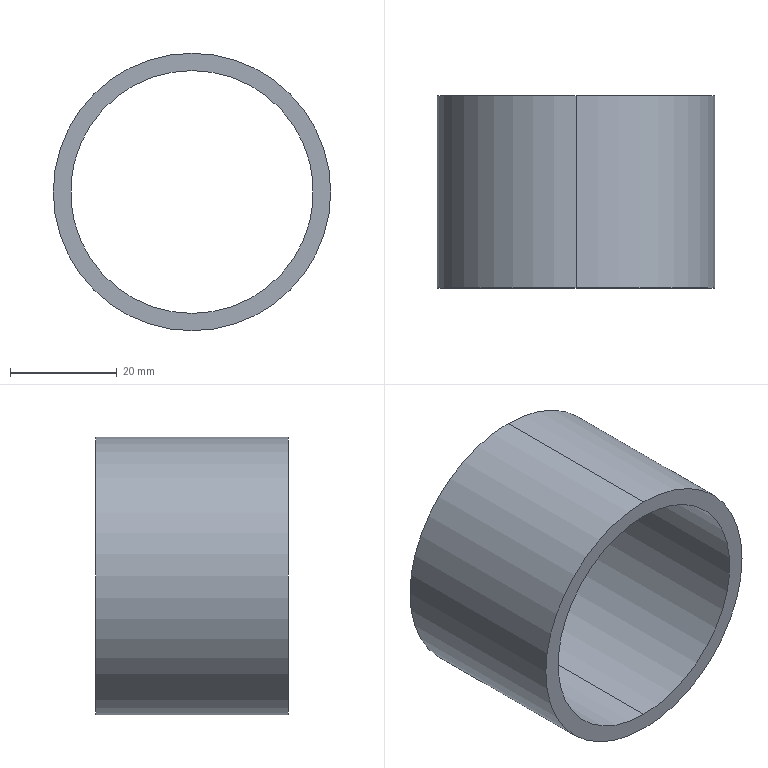Part | STEP file | bearing spacer_default | 1 solid | 6 faces | box 52 x 36 x 52 mm | volume 17919 mm3 | cylinder 4 | plane 2 | commonest cylinder face diameters 45.5 x2 52 x2
STEP:
#1=CARTESIAN_POINT('',(0.,0.,0.));
#2=DIRECTION('',(0.,0.,1.));
#3=DIRECTION('',(1.,0.,0.));
#4=AXIS2_PLACEMENT_3D('',#1,#2,#3);
#5=CARTESIAN_POINT('',(0.,36.,-22.75));
#6=VERTEX_POINT('',#5);
#7=CARTESIAN_POINT('',(0.,0.,-22.75));
#8=VERTEX_POINT('',#7);
#9=CARTESIAN_POINT('',(0.,36.,-22.75));
#10=DIRECTION('',(0.,-1.,0.));
#11=VECTOR('',#10,1.);
#12=LINE('',#9,#11);
#13=CARTESIAN_POINT('',(0.,36.,0.));
#14=DIRECTION('',(0.,-1.,0.));
#15=DIRECTION('',(0.,0.,-1.));
#16=AXIS2_PLACEMENT_3D('',#13,#14,#15);
#17=CYLINDRICAL_SURFACE('',#16,22.75);
#18=CARTESIAN_POINT('',(6.283,0.));
#19=DIRECTION('',(0.,1.));
#20=VECTOR('',#19,1.);
#21=LINE('',#18,#20);
#22=(GEOMETRIC_REPRESENTATION_CONTEXT(2)PARAMETRIC_REPRESENTATION_CONTEXT()REPRESENTATION_CONTEXT('',''));
#23=DEFINITIONAL_REPRESENTATION('',(#21),#22);
#24=PCURVE('',#17,#23);
#25=CARTESIAN_POINT('',(0.,36.,0.));
#26=DIRECTION('',(0.,-1.,0.));
#27=DIRECTION('',(0.,0.,-1.));
#28=AXIS2_PLACEMENT_3D('',#25,#26,#27);
#29=CYLINDRICAL_SURFACE('',#28,22.75);
#30=CARTESIAN_POINT('',(0.,0.));
#31=DIRECTION('',(0.,1.));
#32=VECTOR('',#31,1.);
#33=LINE('',#30,#32);
#34=(GEOMETRIC_REPRESENTATION_CONTEXT(2)PARAMETRIC_REPRESENTATION_CONTEXT()REPRESENTATION_CONTEXT('',''));
#35=DEFINITIONAL_REPRESENTATION('',(#33),#34);
#36=PCURVE('',#29,#35);
#37=SURFACE_CURVE('',#12,(#24,#36),.PCURVE_S1.);
#38=EDGE_CURVE('',#6,#8,#37,.T.);
#39=ORIENTED_EDGE('',*,*,#38,.T.);
#40=CARTESIAN_POINT('',(0.,0.,22.75));
#41=VERTEX_POINT('',#40);
#42=CARTESIAN_POINT('',(0.,0.,0.));
#43=DIRECTION('',(0.,1.,0.));
#44=DIRECTION('',(0.,0.,1.));
#45=AXIS2_PLACEMENT_3D('',#42,#43,#44);
#46=CIRCLE('',#45,22.75);
#47=CARTESIAN_POINT('',(9.425,36.));
#48=DIRECTION('',(-1.,0.));
#49=VECTOR('',#48,1.);
#50=LINE('',#47,#49);
#51=(GEOMETRIC_REPRESENTATION_CONTEXT(2)PARAMETRIC_REPRESENTATION_CONTEXT()REPRESENTATION_CONTEXT('',''));
#52=DEFINITIONAL_REPRESENTATION('',(#50),#51);
#53=PCURVE('',#17,#52);
#54=CARTESIAN_POINT('',(0.,0.,0.));
#55=DIRECTION('',(0.,1.,0.));
#56=DIRECTION('',(0.,0.,1.));
#57=AXIS2_PLACEMENT_3D('',#54,#55,#56);
#58=PLANE('',#57);
#59=CARTESIAN_POINT('',(0.,0.));
#60=DIRECTION('',(1.,0.));
#61=AXIS2_PLACEMENT_2D('',#59,#60);
#62=CIRCLE('',#61,22.75);
#63=(GEOMETRIC_REPRESENTATION_CONTEXT(2)PARAMETRIC_REPRESENTATION_CONTEXT()REPRESENTATION_CONTEXT('',''));
#64=DEFINITIONAL_REPRESENTATION('',(#62),#63);
#65=PCURVE('',#58,#64);
#66=SURFACE_CURVE('',#46,(#53,#65),.PCURVE_S1.);
#67=EDGE_CURVE('',#8,#41,#66,.T.);
#68=ORIENTED_EDGE('',*,*,#67,.T.);
#69=CARTESIAN_POINT('',(0.,36.,22.75));
#70=VERTEX_POINT('',#69);
#71=CARTESIAN_POINT('',(0.,36.,22.75));
#72=DIRECTION('',(0.,-1.,0.));
#73=VECTOR('',#72,1.);
#74=LINE('',#71,#73);
#75=CARTESIAN_POINT('',(3.142,0.));
#76=DIRECTION('',(0.,1.));
#77=VECTOR('',#76,1.);
#78=LINE('',#75,#77);
#79=(GEOMETRIC_REPRESENTATION_CONTEXT(2)PARAMETRIC_REPRESENTATION_CONTEXT()REPRESENTATION_CONTEXT('',''));
#80=DEFINITIONAL_REPRESENTATION('',(#78),#79);
#81=PCURVE('',#17,#80);
#82=CARTESIAN_POINT('',(3.142,0.));
#83=DIRECTION('',(0.,1.));
#84=VECTOR('',#83,1.);
#85=LINE('',#82,#84);
#86=(GEOMETRIC_REPRESENTATION_CONTEXT(2)PARAMETRIC_REPRESENTATION_CONTEXT()REPRESENTATION_CONTEXT('',''));
#87=DEFINITIONAL_REPRESENTATION('',(#85),#86);
#88=PCURVE('',#29,#87);
#89=SURFACE_CURVE('',#74,(#81,#88),.PCURVE_S1.);
#90=EDGE_CURVE('',#70,#41,#89,.T.);
#91=ORIENTED_EDGE('',*,*,#90,.F.);
#92=CARTESIAN_POINT('',(0.,36.,0.));
#93=DIRECTION('',(0.,1.,0.));
#94=DIRECTION('',(0.,0.,1.));
#95=AXIS2_PLACEMENT_3D('',#92,#93,#94);
#96=CIRCLE('',#95,22.75);
#97=CARTESIAN_POINT('',(9.425,0.));
#98=DIRECTION('',(-1.,0.));
#99=VECTOR('',#98,1.);
#100=LINE('',#97,#99);
#101=(GEOMETRIC_REPRESENTATION_CONTEXT(2)PARAMETRIC_REPRESENTATION_CONTEXT()REPRESENTATION_CONTEXT('',''));
#102=DEFINITIONAL_REPRESENTATION('',(#100),#101);
#103=PCURVE('',#17,#102);
#104=CARTESIAN_POINT('',(0.,36.,0.));
#105=DIRECTION('',(0.,1.,0.));
#106=DIRECTION('',(0.,0.,1.));
#107=AXIS2_PLACEMENT_3D('',#104,#105,#106);
#108=PLANE('',#107);
#109=CARTESIAN_POINT('',(0.,0.));
#110=DIRECTION('',(1.,0.));
#111=AXIS2_PLACEMENT_2D('',#109,#110);
#112=CIRCLE('',#111,22.75);
#113=(GEOMETRIC_REPRESENTATION_CONTEXT(2)PARAMETRIC_REPRESENTATION_CONTEXT()REPRESENTATION_CONTEXT('',''));
#114=DEFINITIONAL_REPRESENTATION('',(#112),#113);
#115=PCURVE('',#108,#114);
#116=SURFACE_CURVE('',#96,(#103,#115),.PCURVE_S1.);
#117=EDGE_CURVE('',#6,#70,#116,.T.);
#118=ORIENTED_EDGE('',*,*,#117,.F.);
#119=EDGE_LOOP('',(#39,#68,#91,#118));
#120=FACE_BOUND('',#119,.F.);
#121=ADVANCED_FACE('',(#120),#17,.F.);
#122=CARTESIAN_POINT('',(0.,36.,26.));
#123=VERTEX_POINT('',#122);
#124=CARTESIAN_POINT('',(0.,36.,-26.));
#125=VERTEX_POINT('',#124);
#126=CARTESIAN_POINT('',(0.,36.,0.));
#127=DIRECTION('',(0.,1.,0.));
#128=DIRECTION('',(0.,0.,1.));
#129=AXIS2_PLACEMENT_3D('',#126,#127,#128);
#130=CIRCLE('',#129,26.);
#131=CARTESIAN_POINT('',(0.,36.,0.));
#132=DIRECTION('',(0.,-1.,0.));
#133=DIRECTION('',(0.,0.,-1.));
#134=AXIS2_PLACEMENT_3D('',#131,#132,#133);
#135=CYLINDRICAL_SURFACE('',#134,26.);
#136=CARTESIAN_POINT('',(3.142,0.));
#137=DIRECTION('',(-1.,0.));
#138=VECTOR('',#137,1.);
#139=LINE('',#136,#138);
#140=(GEOMETRIC_REPRESENTATION_CONTEXT(2)PARAMETRIC_REPRESENTATION_CONTEXT()REPRESENTATION_CONTEXT('',''));
#141=DEFINITIONAL_REPRESENTATION('',(#139),#140);
#142=PCURVE('',#135,#141);
#143=CARTESIAN_POINT('',(0.,0.));
#144=DIRECTION('',(1.,0.));
#145=AXIS2_PLACEMENT_2D('',#143,#144);
#146=CIRCLE('',#145,26.);
#147=(GEOMETRIC_REPRESENTATION_CONTEXT(2)PARAMETRIC_REPRESENTATION_CONTEXT()REPRESENTATION_CONTEXT('',''));
#148=DEFINITIONAL_REPRESENTATION('',(#146),#147);
#149=PCURVE('',#108,#148);
#150=SURFACE_CURVE('',#130,(#142,#149),.PCURVE_S1.);
#151=EDGE_CURVE('',#123,#125,#150,.T.);
#152=ORIENTED_EDGE('',*,*,#151,.F.);
#153=CARTESIAN_POINT('',(0.,0.,26.));
#154=VERTEX_POINT('',#153);
#155=CARTESIAN_POINT('',(0.,36.,26.));
#156=DIRECTION('',(0.,-1.,0.));
#157=VECTOR('',#156,1.);
#158=LINE('',#155,#157);
#159=CARTESIAN_POINT('',(3.142,0.));
#160=DIRECTION('',(0.,1.));
#161=VECTOR('',#160,1.);
#162=LINE('',#159,#161);
#163=(GEOMETRIC_REPRESENTATION_CONTEXT(2)PARAMETRIC_REPRESENTATION_CONTEXT()REPRESENTATION_CONTEXT('',''));
#164=DEFINITIONAL_REPRESENTATION('',(#162),#163);
#165=PCURVE('',#135,#164);
#166=CARTESIAN_POINT('',(0.,36.,0.));
#167=DIRECTION('',(0.,-1.,0.));
#168=DIRECTION('',(0.,0.,-1.));
#169=AXIS2_PLACEMENT_3D('',#166,#167,#168);
#170=CYLINDRICAL_SURFACE('',#169,26.);
#171=CARTESIAN_POINT('',(3.142,0.));
#172=DIRECTION('',(0.,1.));
#173=VECTOR('',#172,1.);
#174=LINE('',#171,#173);
#175=(GEOMETRIC_REPRESENTATION_CONTEXT(2)PARAMETRIC_REPRESENTATION_CONTEXT()REPRESENTATION_CONTEXT('',''));
#176=DEFINITIONAL_REPRESENTATION('',(#174),#175);
#177=PCURVE('',#170,#176);
#178=SURFACE_CURVE('',#158,(#165,#177),.PCURVE_S1.);
#179=EDGE_CURVE('',#123,#154,#178,.T.);
#180=ORIENTED_EDGE('',*,*,#179,.T.);
#181=CARTESIAN_POINT('',(0.,0.,-26.));
#182=VERTEX_POINT('',#181);
#183=CARTESIAN_POINT('',(0.,0.,0.));
#184=DIRECTION('',(0.,1.,0.));
#185=DIRECTION('',(0.,0.,1.));
#186=AXIS2_PLACEMENT_3D('',#183,#184,#185);
#187=CIRCLE('',#186,26.);
#188=CARTESIAN_POINT('',(3.142,36.));
#189=DIRECTION('',(-1.,0.));
#190=VECTOR('',#189,1.);
#191=LINE('',#188,#190);
#192=(GEOMETRIC_REPRESENTATION_CONTEXT(2)PARAMETRIC_REPRESENTATION_CONTEXT()REPRESENTATION_CONTEXT('',''));
#193=DEFINITIONAL_REPRESENTATION('',(#191),#192);
#194=PCURVE('',#135,#193);
#195=CARTESIAN_POINT('',(0.,0.));
#196=DIRECTION('',(1.,0.));
#197=AXIS2_PLACEMENT_2D('',#195,#196);
#198=CIRCLE('',#197,26.);
#199=(GEOMETRIC_REPRESENTATION_CONTEXT(2)PARAMETRIC_REPRESENTATION_CONTEXT()REPRESENTATION_CONTEXT('',''));
#200=DEFINITIONAL_REPRESENTATION('',(#198),#199);
#201=PCURVE('',#58,#200);
#202=SURFACE_CURVE('',#187,(#194,#201),.PCURVE_S1.);
#203=EDGE_CURVE('',#154,#182,#202,.T.);
#204=ORIENTED_EDGE('',*,*,#203,.T.);
#205=CARTESIAN_POINT('',(0.,36.,-26.));
#206=DIRECTION('',(0.,-1.,0.));
#207=VECTOR('',#206,1.);
#208=LINE('',#205,#207);
#209=CARTESIAN_POINT('',(0.,0.));
#210=DIRECTION('',(0.,1.));
#211=VECTOR('',#210,1.);
#212=LINE('',#209,#211);
#213=(GEOMETRIC_REPRESENTATION_CONTEXT(2)PARAMETRIC_REPRESENTATION_CONTEXT()REPRESENTATION_CONTEXT('',''));
#214=DEFINITIONAL_REPRESENTATION('',(#212),#213);
#215=PCURVE('',#135,#214);
#216=CARTESIAN_POINT('',(6.283,0.));
#217=DIRECTION('',(0.,1.));
#218=VECTOR('',#217,1.);
#219=LINE('',#216,#218);
#220=(GEOMETRIC_REPRESENTATION_CONTEXT(2)PARAMETRIC_REPRESENTATION_CONTEXT()REPRESENTATION_CONTEXT('',''));
#221=DEFINITIONAL_REPRESENTATION('',(#219),#220);
#222=PCURVE('',#170,#221);
#223=SURFACE_CURVE('',#208,(#215,#222),.PCURVE_S1.);
#224=EDGE_CURVE('',#125,#182,#223,.T.);
#225=ORIENTED_EDGE('',*,*,#224,.F.);
#226=EDGE_LOOP('',(#152,#180,#204,#225));
#227=FACE_BOUND('',#226,.T.);
#228=ADVANCED_FACE('',(#227),#135,.T.);
#229=CARTESIAN_POINT('',(0.,36.,0.));
#230=DIRECTION('',(0.,1.,0.));
#231=DIRECTION('',(0.,0.,1.));
#232=AXIS2_PLACEMENT_3D('',#229,#230,#231);
#233=CIRCLE('',#232,26.);
#234=CARTESIAN_POINT('',(0.,0.));
#235=DIRECTION('',(1.,0.));
#236=AXIS2_PLACEMENT_2D('',#234,#235);
#237=CIRCLE('',#236,26.);
#238=(GEOMETRIC_REPRESENTATION_CONTEXT(2)PARAMETRIC_REPRESENTATION_CONTEXT()REPRESENTATION_CONTEXT('',''));
#239=DEFINITIONAL_REPRESENTATION('',(#237),#238);
#240=PCURVE('',#108,#239);
#241=CARTESIAN_POINT('',(9.425,0.));
#242=DIRECTION('',(-1.,0.));
#243=VECTOR('',#242,1.);
#244=LINE('',#241,#243);
#245=(GEOMETRIC_REPRESENTATION_CONTEXT(2)PARAMETRIC_REPRESENTATION_CONTEXT()REPRESENTATION_CONTEXT('',''));
#246=DEFINITIONAL_REPRESENTATION('',(#244),#245);
#247=PCURVE('',#170,#246);
#248=SURFACE_CURVE('',#233,(#240,#247),.PCURVE_S1.);
#249=EDGE_CURVE('',#125,#123,#248,.T.);
#250=ORIENTED_EDGE('',*,*,#249,.T.);
#251=ORIENTED_EDGE('',*,*,#151,.T.);
#252=EDGE_LOOP('',(#250,#251));
#253=FACE_BOUND('',#252,.T.);
#254=ORIENTED_EDGE('',*,*,#117,.F.);
#255=CARTESIAN_POINT('',(0.,36.,0.));
#256=DIRECTION('',(0.,1.,0.));
#257=DIRECTION('',(0.,0.,1.));
#258=AXIS2_PLACEMENT_3D('',#255,#256,#257);
#259=CIRCLE('',#258,22.75);
#260=CARTESIAN_POINT('',(0.,0.));
#261=DIRECTION('',(1.,0.));
#262=AXIS2_PLACEMENT_2D('',#260,#261);
#263=CIRCLE('',#262,22.75);
#264=(GEOMETRIC_REPRESENTATION_CONTEXT(2)PARAMETRIC_REPRESENTATION_CONTEXT()REPRESENTATION_CONTEXT('',''));
#265=DEFINITIONAL_REPRESENTATION('',(#263),#264);
#266=PCURVE('',#108,#265);
#267=CARTESIAN_POINT('',(3.142,0.));
#268=DIRECTION('',(-1.,0.));
#269=VECTOR('',#268,1.);
#270=LINE('',#267,#269);
#271=(GEOMETRIC_REPRESENTATION_CONTEXT(2)PARAMETRIC_REPRESENTATION_CONTEXT()REPRESENTATION_CONTEXT('',''));
#272=DEFINITIONAL_REPRESENTATION('',(#270),#271);
#273=PCURVE('',#29,#272);
#274=SURFACE_CURVE('',#259,(#266,#273),.PCURVE_S1.);
#275=EDGE_CURVE('',#70,#6,#274,.T.);
#276=ORIENTED_EDGE('',*,*,#275,.F.);
#277=EDGE_LOOP('',(#254,#276));
#278=FACE_BOUND('',#277,.T.);
#279=ADVANCED_FACE('',(#253,#278),#108,.T.);
#280=CARTESIAN_POINT('',(0.,0.,0.));
#281=DIRECTION('',(0.,1.,0.));
#282=DIRECTION('',(0.,0.,1.));
#283=AXIS2_PLACEMENT_3D('',#280,#281,#282);
#284=CIRCLE('',#283,26.);
#285=CARTESIAN_POINT('',(0.,0.));
#286=DIRECTION('',(1.,0.));
#287=AXIS2_PLACEMENT_2D('',#285,#286);
#288=CIRCLE('',#287,26.);
#289=(GEOMETRIC_REPRESENTATION_CONTEXT(2)PARAMETRIC_REPRESENTATION_CONTEXT()REPRESENTATION_CONTEXT('',''));
#290=DEFINITIONAL_REPRESENTATION('',(#288),#289);
#291=PCURVE('',#58,#290);
#292=CARTESIAN_POINT('',(9.425,36.));
#293=DIRECTION('',(-1.,0.));
#294=VECTOR('',#293,1.);
#295=LINE('',#292,#294);
#296=(GEOMETRIC_REPRESENTATION_CONTEXT(2)PARAMETRIC_REPRESENTATION_CONTEXT()REPRESENTATION_CONTEXT('',''));
#297=DEFINITIONAL_REPRESENTATION('',(#295),#296);
#298=PCURVE('',#170,#297);
#299=SURFACE_CURVE('',#284,(#291,#298),.PCURVE_S1.);
#300=EDGE_CURVE('',#182,#154,#299,.T.);
#301=ORIENTED_EDGE('',*,*,#300,.F.);
#302=ORIENTED_EDGE('',*,*,#203,.F.);
#303=EDGE_LOOP('',(#301,#302));
#304=FACE_BOUND('',#303,.T.);
#305=ORIENTED_EDGE('',*,*,#67,.T.);
#306=CARTESIAN_POINT('',(0.,0.,0.));
#307=DIRECTION('',(0.,1.,0.));
#308=DIRECTION('',(0.,0.,1.));
#309=AXIS2_PLACEMENT_3D('',#306,#307,#308);
#310=CIRCLE('',#309,22.75);
#311=CARTESIAN_POINT('',(0.,0.));
#312=DIRECTION('',(1.,0.));
#313=AXIS2_PLACEMENT_2D('',#311,#312);
#314=CIRCLE('',#313,22.75);
#315=(GEOMETRIC_REPRESENTATION_CONTEXT(2)PARAMETRIC_REPRESENTATION_CONTEXT()REPRESENTATION_CONTEXT('',''));
#316=DEFINITIONAL_REPRESENTATION('',(#314),#315);
#317=PCURVE('',#58,#316);
#318=CARTESIAN_POINT('',(3.142,36.));
#319=DIRECTION('',(-1.,0.));
#320=VECTOR('',#319,1.);
#321=LINE('',#318,#320);
#322=(GEOMETRIC_REPRESENTATION_CONTEXT(2)PARAMETRIC_REPRESENTATION_CONTEXT()REPRESENTATION_CONTEXT('',''));
#323=DEFINITIONAL_REPRESENTATION('',(#321),#322);
#324=PCURVE('',#29,#323);
#325=SURFACE_CURVE('',#310,(#317,#324),.PCURVE_S1.);
#326=EDGE_CURVE('',#41,#8,#325,.T.);
#327=ORIENTED_EDGE('',*,*,#326,.T.);
#328=EDGE_LOOP('',(#305,#327));
#329=FACE_BOUND('',#328,.T.);
#330=ADVANCED_FACE('',(#304,#329),#58,.F.);
#331=ORIENTED_EDGE('',*,*,#179,.F.);
#332=ORIENTED_EDGE('',*,*,#249,.F.);
#333=ORIENTED_EDGE('',*,*,#224,.T.);
#334=ORIENTED_EDGE('',*,*,#300,.T.);
#335=EDGE_LOOP('',(#331,#332,#333,#334));
#336=FACE_BOUND('',#335,.T.);
#337=ADVANCED_FACE('',(#336),#170,.T.);
#338=ORIENTED_EDGE('',*,*,#326,.T.);
#339=ORIENTED_EDGE('',*,*,#38,.F.);
#340=ORIENTED_EDGE('',*,*,#275,.F.);
#341=ORIENTED_EDGE('',*,*,#90,.T.);
#342=EDGE_LOOP('',(#338,#339,#340,#341));
#343=FACE_BOUND('',#342,.F.);
#344=ADVANCED_FACE('',(#343),#29,.F.);
#345=CLOSED_SHELL('',(#121,#228,#279,#330,#337,#344));
#346=MANIFOLD_SOLID_BREP('',#345);
#347=(LENGTH_UNIT()NAMED_UNIT(*)SI_UNIT(.MILLI.,.METRE.));
#348=UNCERTAINTY_MEASURE_WITH_UNIT(LENGTH_MEASURE(0.0000001),#347,'','');
#349=(NAMED_UNIT(*)PLANE_ANGLE_UNIT()SI_UNIT($,.RADIAN.));
#350=(NAMED_UNIT(*)SI_UNIT($,.STERADIAN.)SOLID_ANGLE_UNIT());
#351=(GEOMETRIC_REPRESENTATION_CONTEXT(3)GLOBAL_UNCERTAINTY_ASSIGNED_CONTEXT((#348))GLOBAL_UNIT_ASSIGNED_CONTEXT((#347,#349,#350))REPRESENTATION_CONTEXT('',''));
#352=ADVANCED_BREP_SHAPE_REPRESENTATION('',(#4,#346),#351);